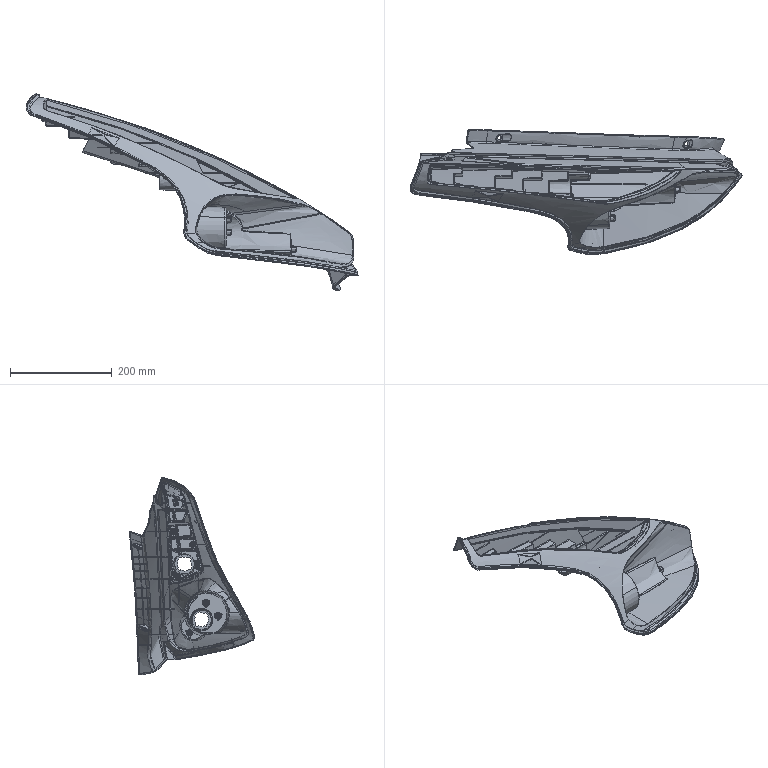Part | STEP file | solid 275 | 1 solid | 1833 faces | box 652.466 x 245.902 x 388.968 mm | volume 649456 mm3 | spline 1384 | plane 196 | sphere 87 | cylinder 72 | torus 44 | cone 41 | other 9 | commonest cylinder face diameters 2.01 x17 4.02 x17 27.135 x8 31.155 x8 2.915 x7 1.005 x6